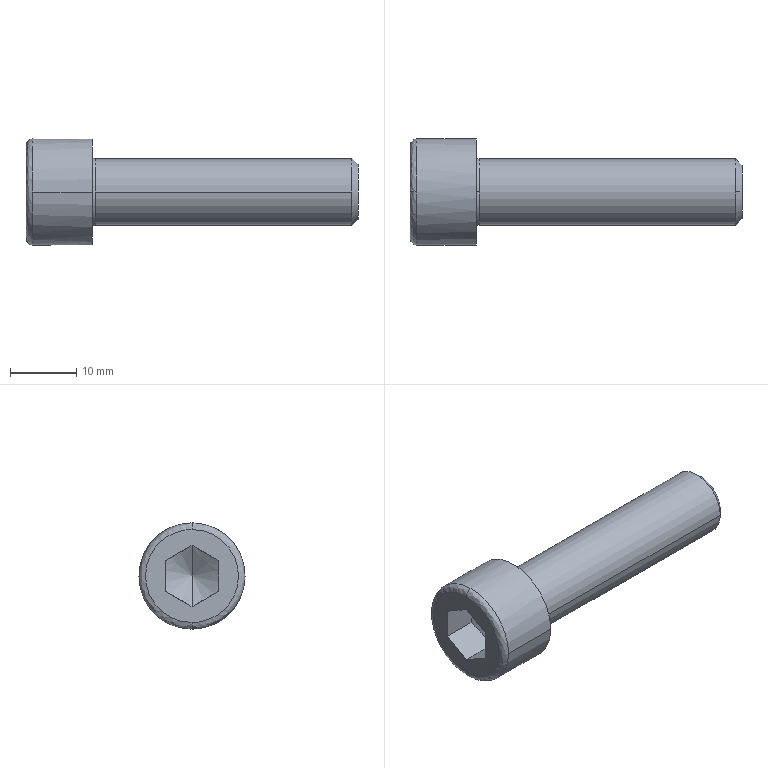Part | STEP file | Broached Socket Head Cap Screw - Metric M10x1.5 x 40 | 1 solid | 21 faces | box 50 x 16 x 16 mm | volume 4795 mm3 | plane 9 | spline 4 | cylinder 4 | cone 4 | commonest cylinder face diameters 10 x2 16 x2